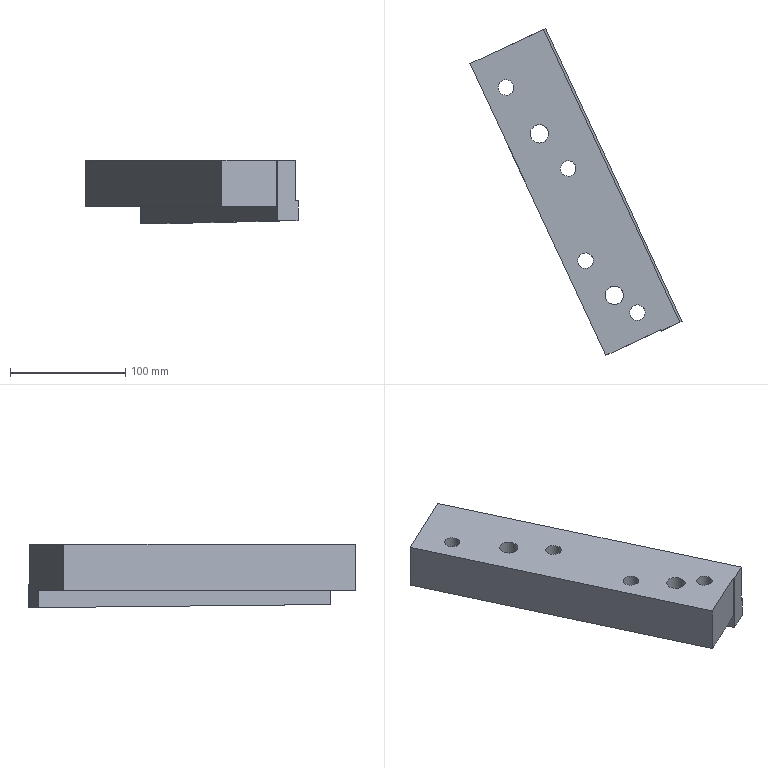Part | NX | features solid 2 | 1 solid | 25 faces | box 183.912 x 283.44 x 55 mm | volume 810388 mm3 | plane 15 | cylinder 10 | commonest cylinder face diameters 13.5 x4 19.5 x4 16 x2
STEP:
#1=CARTESIAN_POINT('',(122.71,137.916,3.));
#2=VERTEX_POINT('',#1);
#3=CARTESIAN_POINT('',(4.8,390.776,3.));
#4=VERTEX_POINT('',#3);
#5=CARTESIAN_POINT('',(204.661,-37.827,3.));
#6=DIRECTION('',(0.4226,-0.9063,0.));
#7=VECTOR('',#6,1000.);
#8=LINE('',#5,#7);
#9=EDGE_CURVE('',#2,#4,#8,.F.);
#10=ORIENTED_EDGE('',*,*,#9,.F.);
#11=CARTESIAN_POINT('',(122.71,137.916,43.));
#12=VERTEX_POINT('',#11);
#13=CARTESIAN_POINT('',(122.71,137.916,-107.));
#14=DIRECTION('',(0.,0.,1.));
#15=VECTOR('',#14,1000.);
#16=LINE('',#13,#15);
#17=EDGE_CURVE('',#2,#12,#16,.T.);
#18=ORIENTED_EDGE('',*,*,#17,.T.);
#19=CARTESIAN_POINT('',(4.8,390.776,43.));
#20=VERTEX_POINT('',#19);
#21=CARTESIAN_POINT('',(192.036,-10.753,43.));
#22=DIRECTION('',(0.4226,-0.9063,0.));
#23=VECTOR('',#22,1000.);
#24=LINE('',#21,#23);
#25=EDGE_CURVE('',#20,#12,#24,.T.);
#26=ORIENTED_EDGE('',*,*,#25,.F.);
#27=CARTESIAN_POINT('',(4.8,390.776,-107.));
#28=DIRECTION('',(0.,0.,-1.));
#29=VECTOR('',#28,1000.);
#30=LINE('',#27,#29);
#31=EDGE_CURVE('',#4,#20,#30,.F.);
#32=ORIENTED_EDGE('',*,*,#31,.F.);
#33=EDGE_LOOP('',(#10,#18,#26,#32));
#34=FACE_BOUND('',#33,.T.);
#35=CARTESIAN_POINT('',(215.,-60.,-107.));
#36=DIRECTION('',(-0.9063,-0.4226,0.));
#37=DIRECTION('',(-0.4226,0.9063,0.));
#38=AXIS2_PLACEMENT_3D('',#35,#36,#37);
#39=PLANE('',#38);
#40=ADVANCED_FACE('',(#34),#39,.T.);
#41=CARTESIAN_POINT('',(70.379,421.356,-12.));
#42=VERTEX_POINT('',#41);
#43=CARTESIAN_POINT('',(70.379,421.356,8.));
#44=VERTEX_POINT('',#43);
#45=CARTESIAN_POINT('',(70.379,421.356,-105.));
#46=DIRECTION('',(0.,0.,-1.));
#47=VECTOR('',#46,1000.);
#48=LINE('',#45,#47);
#49=EDGE_CURVE('',#42,#44,#48,.F.);
#50=ORIENTED_EDGE('',*,*,#49,.F.);
#51=CARTESIAN_POINT('',(52.252,412.903,-11.91));
#52=VERTEX_POINT('',#51);
#53=CARTESIAN_POINT('',(70.35,421.342,-12.));
#54=DIRECTION('',(-0.9063,-0.4226,0.004484));
#55=VECTOR('',#54,1000.);
#56=LINE('',#53,#55);
#57=EDGE_CURVE('',#42,#52,#56,.T.);
#58=ORIENTED_EDGE('',*,*,#57,.T.);
#59=CARTESIAN_POINT('',(52.252,412.903,3.));
#60=VERTEX_POINT('',#59);
#61=CARTESIAN_POINT('',(52.252,412.903,-5.));
#62=DIRECTION('',(0.,0.,1.));
#63=VECTOR('',#62,1000.);
#64=LINE('',#61,#63);
#65=EDGE_CURVE('',#60,#52,#64,.F.);
#66=ORIENTED_EDGE('',*,*,#65,.F.);
#67=CARTESIAN_POINT('',(-49.65,365.386,3.));
#68=DIRECTION('',(0.9063,0.4226,0.));
#69=VECTOR('',#68,1000.);
#70=LINE('',#67,#69);
#71=EDGE_CURVE('',#4,#60,#70,.T.);
#72=ORIENTED_EDGE('',*,*,#71,.F.);
#73=ORIENTED_EDGE('',*,*,#31,.T.);
#74=CARTESIAN_POINT('',(68.566,420.51,43.));
#75=VERTEX_POINT('',#74);
#76=CARTESIAN_POINT('',(204.565,483.928,43.));
#77=DIRECTION('',(0.9063,0.4226,0.));
#78=VECTOR('',#77,1000.);
#79=LINE('',#76,#78);
#80=EDGE_CURVE('',#20,#75,#79,.T.);
#81=ORIENTED_EDGE('',*,*,#80,.T.);
#82=CARTESIAN_POINT('',(68.566,420.51,8.));
#83=VERTEX_POINT('',#82);
#84=CARTESIAN_POINT('',(68.566,420.51,43.));
#85=DIRECTION('',(0.,0.,-1.));
#86=VECTOR('',#85,1000.);
#87=LINE('',#84,#86);
#88=EDGE_CURVE('',#83,#75,#87,.F.);
#89=ORIENTED_EDGE('',*,*,#88,.F.);
#90=CARTESIAN_POINT('',(-32.617,373.328,8.));
#91=DIRECTION('',(-0.9063,-0.4226,0.));
#92=VECTOR('',#91,1000.);
#93=LINE('',#90,#92);
#94=EDGE_CURVE('',#44,#83,#93,.T.);
#95=ORIENTED_EDGE('',*,*,#94,.F.);
#96=EDGE_LOOP('',(#50,#58,#66,#72,#73,#81,#89,#95));
#97=FACE_BOUND('',#96,.T.);
#98=CARTESIAN_POINT('',(70.379,421.356,-5.));
#99=DIRECTION('',(-0.4226,0.9063,0.));
#100=DIRECTION('',(0.,0.,-1.));
#101=AXIS2_PLACEMENT_3D('',#98,#99,#100);
#102=PLANE('',#101);
#103=ADVANCED_FACE('',(#97),#102,.T.);
#104=CARTESIAN_POINT('',(186.899,166.744,8.));
#105=VERTEX_POINT('',#104);
#106=CARTESIAN_POINT('',(81.245,393.321,8.));
#107=DIRECTION('',(-0.4226,0.9063,0.));
#108=VECTOR('',#107,1000.);
#109=LINE('',#106,#108);
#110=EDGE_CURVE('',#83,#105,#109,.F.);
#111=ORIENTED_EDGE('',*,*,#110,.F.);
#112=ORIENTED_EDGE('',*,*,#88,.T.);
#113=CARTESIAN_POINT('',(186.899,166.744,43.));
#114=VERTEX_POINT('',#113);
#115=CARTESIAN_POINT('',(81.245,393.321,43.));
#116=DIRECTION('',(-0.4226,0.9063,0.));
#117=VECTOR('',#116,1000.);
#118=LINE('',#115,#117);
#119=EDGE_CURVE('',#75,#114,#118,.F.);
#120=ORIENTED_EDGE('',*,*,#119,.T.);
#121=CARTESIAN_POINT('',(186.899,166.744,43.));
#122=DIRECTION('',(0.,0.,1.));
#123=VECTOR('',#122,1000.);
#124=LINE('',#121,#123);
#125=EDGE_CURVE('',#105,#114,#124,.T.);
#126=ORIENTED_EDGE('',*,*,#125,.F.);
#127=EDGE_LOOP('',(#111,#112,#120,#126));
#128=FACE_BOUND('',#127,.T.);
#129=CARTESIAN_POINT('',(81.245,393.321,43.));
#130=DIRECTION('',(-0.9063,-0.4226,0.));
#131=DIRECTION('',(-0.4226,0.9063,0.));
#132=AXIS2_PLACEMENT_3D('',#129,#130,#131);
#133=PLANE('',#132);
#134=ADVANCED_FACE('',(#128),#133,.F.);
#135=CARTESIAN_POINT('',(188.712,167.589,-9.308));
#136=VERTEX_POINT('',#135);
#137=CARTESIAN_POINT('',(281.198,-30.747,-7.203));
#138=DIRECTION('',(-0.4226,0.9063,-0.009616));
#139=VECTOR('',#138,1000.);
#140=LINE('',#137,#139);
#141=EDGE_CURVE('',#42,#136,#140,.F.);
#142=ORIENTED_EDGE('',*,*,#141,.F.);
#143=ORIENTED_EDGE('',*,*,#49,.T.);
#144=CARTESIAN_POINT('',(188.712,167.589,8.));
#145=VERTEX_POINT('',#144);
#146=CARTESIAN_POINT('',(178.495,189.499,8.));
#147=DIRECTION('',(-0.4226,0.9063,0.));
#148=VECTOR('',#147,1000.);
#149=LINE('',#146,#148);
#150=EDGE_CURVE('',#44,#145,#149,.F.);
#151=ORIENTED_EDGE('',*,*,#150,.T.);
#152=CARTESIAN_POINT('',(188.712,167.589,-105.));
#153=DIRECTION('',(0.,0.,1.));
#154=VECTOR('',#153,1000.);
#155=LINE('',#152,#154);
#156=EDGE_CURVE('',#136,#145,#155,.T.);
#157=ORIENTED_EDGE('',*,*,#156,.F.);
#158=EDGE_LOOP('',(#142,#143,#151,#157));
#159=FACE_BOUND('',#158,.T.);
#160=CARTESIAN_POINT('',(290.14,-49.924,-105.));
#161=DIRECTION('',(-0.9063,-0.4226,0.));
#162=DIRECTION('',(-0.4226,0.9063,0.));
#163=AXIS2_PLACEMENT_3D('',#160,#161,#162);
#164=PLANE('',#163);
#165=ADVANCED_FACE('',(#159),#164,.F.);
#166=ORIENTED_EDGE('',*,*,#150,.F.);
#167=ORIENTED_EDGE('',*,*,#94,.T.);
#168=ORIENTED_EDGE('',*,*,#110,.T.);
#169=CARTESIAN_POINT('',(85.717,119.562,8.));
#170=DIRECTION('',(0.9063,0.4226,0.));
#171=VECTOR('',#170,1000.);
#172=LINE('',#169,#171);
#173=EDGE_CURVE('',#145,#105,#172,.F.);
#174=ORIENTED_EDGE('',*,*,#173,.F.);
#175=EDGE_LOOP('',(#166,#167,#168,#174));
#176=FACE_BOUND('',#175,.T.);
#177=CARTESIAN_POINT('',(-40.145,389.473,8.));
#178=DIRECTION('',(0.,0.,1.));
#179=DIRECTION('',(0.08716,-0.9962,0.));
#180=AXIS2_PLACEMENT_3D('',#177,#178,#179);
#181=PLANE('',#180);
#182=ADVANCED_FACE('',(#176),#181,.T.);
#183=CARTESIAN_POINT('',(170.586,159.137,-9.218));
#184=VERTEX_POINT('',#183);
#185=CARTESIAN_POINT('',(170.586,159.137,43.));
#186=VERTEX_POINT('',#185);
#187=CARTESIAN_POINT('',(170.586,159.137,3.));
#188=DIRECTION('',(0.,0.,1.));
#189=VECTOR('',#188,1000.);
#190=LINE('',#187,#189);
#191=EDGE_CURVE('',#184,#186,#190,.T.);
#192=ORIENTED_EDGE('',*,*,#191,.T.);
#193=CARTESIAN_POINT('',(170.163,160.043,43.));
#194=VERTEX_POINT('',#193);
#195=CARTESIAN_POINT('',(64.931,385.714,43.));
#196=DIRECTION('',(0.4226,-0.9063,0.));
#197=VECTOR('',#196,1000.);
#198=LINE('',#195,#197);
#199=EDGE_CURVE('',#194,#186,#198,.T.);
#200=ORIENTED_EDGE('',*,*,#199,.F.);
#201=CARTESIAN_POINT('',(170.163,160.043,3.));
#202=VERTEX_POINT('',#201);
#203=CARTESIAN_POINT('',(170.163,160.043,3.));
#204=DIRECTION('',(0.,0.,-1.));
#205=VECTOR('',#204,1000.);
#206=LINE('',#203,#205);
#207=EDGE_CURVE('',#202,#194,#206,.F.);
#208=ORIENTED_EDGE('',*,*,#207,.F.);
#209=CARTESIAN_POINT('',(64.931,385.714,3.));
#210=DIRECTION('',(0.4226,-0.9063,0.));
#211=VECTOR('',#210,1000.);
#212=LINE('',#209,#211);
#213=EDGE_CURVE('',#60,#202,#212,.T.);
#214=ORIENTED_EDGE('',*,*,#213,.F.);
#215=ORIENTED_EDGE('',*,*,#65,.T.);
#216=CARTESIAN_POINT('',(263.071,-39.199,-7.114));
#217=DIRECTION('',(-0.4226,0.9063,-0.009616));
#218=VECTOR('',#217,1000.);
#219=LINE('',#216,#218);
#220=EDGE_CURVE('',#52,#184,#219,.F.);
#221=ORIENTED_EDGE('',*,*,#220,.T.);
#222=EDGE_LOOP('',(#192,#200,#208,#214,#215,#221));
#223=FACE_BOUND('',#222,.T.);
#224=CARTESIAN_POINT('',(64.931,385.714,3.));
#225=DIRECTION('',(-0.9063,-0.4226,0.));
#226=DIRECTION('',(-0.4226,0.9063,0.));
#227=AXIS2_PLACEMENT_3D('',#224,#225,#226);
#228=PLANE('',#227);
#229=ADVANCED_FACE('',(#223),#228,.T.);
#230=CARTESIAN_POINT('',(65.,322.,3.));
#231=VERTEX_POINT('',#230);
#232=CARTESIAN_POINT('',(65.,330.,3.));
#233=DIRECTION('',(0.,0.,-1.));
#234=DIRECTION('',(0.,-1.,0.));
#235=AXIS2_PLACEMENT_3D('',#232,#233,#234);
#236=CIRCLE('',#235,8.);
#237=EDGE_CURVE('',#231,#231,#236,.T.);
#238=ORIENTED_EDGE('',*,*,#237,.F.);
#239=EDGE_LOOP('',(#238));
#240=FACE_BOUND('',#239,.T.);
#241=CARTESIAN_POINT('',(130.,182.,3.));
#242=VERTEX_POINT('',#241);
#243=CARTESIAN_POINT('',(130.,190.,3.));
#244=DIRECTION('',(0.,0.,-1.));
#245=DIRECTION('',(0.,-1.,0.));
#246=AXIS2_PLACEMENT_3D('',#243,#244,#245);
#247=CIRCLE('',#246,8.);
#248=EDGE_CURVE('',#242,#242,#247,.T.);
#249=ORIENTED_EDGE('',*,*,#248,.F.);
#250=EDGE_LOOP('',(#249));
#251=FACE_BOUND('',#250,.T.);
#252=CARTESIAN_POINT('',(36.079,360.489,3.));
#253=VERTEX_POINT('',#252);
#254=CARTESIAN_POINT('',(36.079,370.239,3.));
#255=DIRECTION('',(0.,0.,-1.));
#256=DIRECTION('',(0.,-1.,0.));
#257=AXIS2_PLACEMENT_3D('',#254,#255,#256);
#258=CIRCLE('',#257,9.75);
#259=EDGE_CURVE('',#253,#253,#258,.T.);
#260=ORIENTED_EDGE('',*,*,#259,.F.);
#261=EDGE_LOOP('',(#260));
#262=FACE_BOUND('',#261,.T.);
#263=CARTESIAN_POINT('',(90.,290.25,3.));
#264=VERTEX_POINT('',#263);
#265=CARTESIAN_POINT('',(90.,300.,3.));
#266=DIRECTION('',(0.,0.,-1.));
#267=DIRECTION('',(0.,-1.,0.));
#268=AXIS2_PLACEMENT_3D('',#265,#266,#267);
#269=CIRCLE('',#268,9.75);
#270=EDGE_CURVE('',#264,#264,#269,.T.);
#271=ORIENTED_EDGE('',*,*,#270,.F.);
#272=EDGE_LOOP('',(#271));
#273=FACE_BOUND('',#272,.T.);
#274=CARTESIAN_POINT('',(105.,210.25,3.));
#275=VERTEX_POINT('',#274);
#276=CARTESIAN_POINT('',(105.,220.,3.));
#277=DIRECTION('',(0.,0.,-1.));
#278=DIRECTION('',(0.,-1.,0.));
#279=AXIS2_PLACEMENT_3D('',#276,#277,#278);
#280=CIRCLE('',#279,9.75);
#281=EDGE_CURVE('',#275,#275,#280,.T.);
#282=ORIENTED_EDGE('',*,*,#281,.F.);
#283=EDGE_LOOP('',(#282));
#284=FACE_BOUND('',#283,.T.);
#285=CARTESIAN_POINT('',(150.,165.25,3.));
#286=VERTEX_POINT('',#285);
#287=CARTESIAN_POINT('',(150.,175.,3.));
#288=DIRECTION('',(0.,0.,-1.));
#289=DIRECTION('',(0.,-1.,0.));
#290=AXIS2_PLACEMENT_3D('',#287,#288,#289);
#291=CIRCLE('',#290,9.75);
#292=EDGE_CURVE('',#286,#286,#291,.T.);
#293=ORIENTED_EDGE('',*,*,#292,.F.);
#294=EDGE_LOOP('',(#293));
#295=FACE_BOUND('',#294,.T.);
#296=ORIENTED_EDGE('',*,*,#213,.T.);
#297=CARTESIAN_POINT('',(123.617,138.339,3.));
#298=DIRECTION('',(0.9063,0.4226,0.));
#299=VECTOR('',#298,1000.);
#300=LINE('',#297,#299);
#301=EDGE_CURVE('',#202,#2,#300,.F.);
#302=ORIENTED_EDGE('',*,*,#301,.T.);
#303=ORIENTED_EDGE('',*,*,#9,.T.);
#304=ORIENTED_EDGE('',*,*,#71,.T.);
#305=EDGE_LOOP('',(#296,#302,#303,#304));
#306=FACE_BOUND('',#305,.T.);
#307=CARTESIAN_POINT('',(-60.069,387.73,3.));
#308=DIRECTION('',(0.,0.,-1.));
#309=DIRECTION('',(0.08716,-0.9962,0.));
#310=AXIS2_PLACEMENT_3D('',#307,#308,#309);
#311=PLANE('',#310);
#312=ADVANCED_FACE('',(#240,#251,#262,#273,#284,#295,#306),#311,.T.);
#313=ORIENTED_EDGE('',*,*,#199,.T.);
#314=CARTESIAN_POINT('',(322.898,230.162,43.));
#315=DIRECTION('',(-0.9063,-0.4226,0.));
#316=VECTOR('',#315,1000.);
#317=LINE('',#314,#316);
#318=EDGE_CURVE('',#186,#114,#317,.F.);
#319=ORIENTED_EDGE('',*,*,#318,.T.);
#320=ORIENTED_EDGE('',*,*,#119,.F.);
#321=ORIENTED_EDGE('',*,*,#80,.F.);
#322=ORIENTED_EDGE('',*,*,#25,.T.);
#323=CARTESIAN_POINT('',(123.617,138.339,43.));
#324=DIRECTION('',(0.9063,0.4226,0.));
#325=VECTOR('',#324,1000.);
#326=LINE('',#323,#325);
#327=EDGE_CURVE('',#194,#12,#326,.F.);
#328=ORIENTED_EDGE('',*,*,#327,.F.);
#329=EDGE_LOOP('',(#313,#319,#320,#321,#322,#328));
#330=FACE_BOUND('',#329,.T.);
#331=CARTESIAN_POINT('',(73.,330.,43.));
#332=VERTEX_POINT('',#331);
#333=CARTESIAN_POINT('',(65.,330.,43.));
#334=DIRECTION('',(0.,0.,1.));
#335=DIRECTION('',(1.,0.,0.));
#336=AXIS2_PLACEMENT_3D('',#333,#334,#335);
#337=CIRCLE('',#336,8.);
#338=EDGE_CURVE('',#332,#332,#337,.F.);
#339=ORIENTED_EDGE('',*,*,#338,.T.);
#340=EDGE_LOOP('',(#339));
#341=FACE_BOUND('',#340,.T.);
#342=CARTESIAN_POINT('',(138.,190.,43.));
#343=VERTEX_POINT('',#342);
#344=CARTESIAN_POINT('',(130.,190.,43.));
#345=DIRECTION('',(0.,0.,1.));
#346=DIRECTION('',(1.,0.,0.));
#347=AXIS2_PLACEMENT_3D('',#344,#345,#346);
#348=CIRCLE('',#347,8.);
#349=EDGE_CURVE('',#343,#343,#348,.F.);
#350=ORIENTED_EDGE('',*,*,#349,.T.);
#351=EDGE_LOOP('',(#350));
#352=FACE_BOUND('',#351,.T.);
#353=CARTESIAN_POINT('',(42.829,370.239,43.));
#354=VERTEX_POINT('',#353);
#355=CARTESIAN_POINT('',(36.079,370.239,43.));
#356=DIRECTION('',(0.,0.,1.));
#357=DIRECTION('',(1.,0.,0.));
#358=AXIS2_PLACEMENT_3D('',#355,#356,#357);
#359=CIRCLE('',#358,6.75);
#360=EDGE_CURVE('',#354,#354,#359,.F.);
#361=ORIENTED_EDGE('',*,*,#360,.T.);
#362=EDGE_LOOP('',(#361));
#363=FACE_BOUND('',#362,.T.);
#364=CARTESIAN_POINT('',(96.75,300.,43.));
#365=VERTEX_POINT('',#364);
#366=CARTESIAN_POINT('',(90.,300.,43.));
#367=DIRECTION('',(0.,0.,1.));
#368=DIRECTION('',(1.,0.,0.));
#369=AXIS2_PLACEMENT_3D('',#366,#367,#368);
#370=CIRCLE('',#369,6.75);
#371=EDGE_CURVE('',#365,#365,#370,.F.);
#372=ORIENTED_EDGE('',*,*,#371,.T.);
#373=EDGE_LOOP('',(#372));
#374=FACE_BOUND('',#373,.T.);
#375=CARTESIAN_POINT('',(111.75,220.,43.));
#376=VERTEX_POINT('',#375);
#377=CARTESIAN_POINT('',(105.,220.,43.));
#378=DIRECTION('',(0.,0.,1.));
#379=DIRECTION('',(1.,0.,0.));
#380=AXIS2_PLACEMENT_3D('',#377,#378,#379);
#381=CIRCLE('',#380,6.75);
#382=EDGE_CURVE('',#376,#376,#381,.F.);
#383=ORIENTED_EDGE('',*,*,#382,.T.);
#384=EDGE_LOOP('',(#383));
#385=FACE_BOUND('',#384,.T.);
#386=CARTESIAN_POINT('',(156.75,175.,43.));
#387=VERTEX_POINT('',#386);
#388=CARTESIAN_POINT('',(150.,175.,43.));
#389=DIRECTION('',(0.,0.,1.));
#390=DIRECTION('',(1.,0.,0.));
#391=AXIS2_PLACEMENT_3D('',#388,#389,#390);
#392=CIRCLE('',#391,6.75);
#393=EDGE_CURVE('',#387,#387,#392,.F.);
#394=ORIENTED_EDGE('',*,*,#393,.T.);
#395=EDGE_LOOP('',(#394));
#396=FACE_BOUND('',#395,.T.);
#397=CARTESIAN_POINT('',(383.563,100.064,43.));
#398=DIRECTION('',(0.,0.,-1.));
#399=DIRECTION('',(0.9962,0.08716,0.));
#400=AXIS2_PLACEMENT_3D('',#397,#398,#399);
#401=PLANE('',#400);
#402=ADVANCED_FACE('',(#330,#341,#352,#363,#374,#385,#396),#401,.F.);
#403=ORIENTED_EDGE('',*,*,#220,.F.);
#404=ORIENTED_EDGE('',*,*,#57,.F.);
#405=ORIENTED_EDGE('',*,*,#141,.T.);
#406=CARTESIAN_POINT('',(155.822,152.253,-9.145));
#407=DIRECTION('',(-0.9063,-0.4226,0.004484));
#408=VECTOR('',#407,1000.);
#409=LINE('',#406,#408);
#410=EDGE_CURVE('',#184,#136,#409,.F.);
#411=ORIENTED_EDGE('',*,*,#410,.F.);
#412=EDGE_LOOP('',(#403,#404,#405,#411));
#413=FACE_BOUND('',#412,.T.);
#414=CARTESIAN_POINT('',(240.127,-49.896,-7.));
#415=DIRECTION('',(0.,-0.01061,-0.9999));
#416=DIRECTION('',(0.,0.9999,-0.01061));
#417=AXIS2_PLACEMENT_3D('',#414,#415,#416);
#418=PLANE('',#417);
#419=ADVANCED_FACE('',(#413),#418,.T.);
#420=ORIENTED_EDGE('',*,*,#318,.F.);
#421=ORIENTED_EDGE('',*,*,#191,.F.);
#422=ORIENTED_EDGE('',*,*,#410,.T.);
#423=ORIENTED_EDGE('',*,*,#156,.T.);
#424=ORIENTED_EDGE('',*,*,#173,.T.);
#425=ORIENTED_EDGE('',*,*,#125,.T.);
#426=EDGE_LOOP('',(#420,#421,#422,#423,#424,#425));
#427=FACE_BOUND('',#426,.T.);
#428=CARTESIAN_POINT('',(155.922,152.3,15.5));
#429=DIRECTION('',(-0.4226,0.9063,0.));
#430=DIRECTION('',(0.9063,0.4226,0.));
#431=AXIS2_PLACEMENT_3D('',#428,#429,#430);
#432=PLANE('',#431);
#433=ADVANCED_FACE('',(#427),#432,.F.);
#434=ORIENTED_EDGE('',*,*,#393,.F.);
#435=EDGE_LOOP('',(#434));
#436=FACE_BOUND('',#435,.T.);
#437=CARTESIAN_POINT('',(150.,168.25,28.));
#438=VERTEX_POINT('',#437);
#439=CARTESIAN_POINT('',(150.,175.,28.));
#440=DIRECTION('',(0.,0.,-1.));
#441=DIRECTION('',(0.,-1.,0.));
#442=AXIS2_PLACEMENT_3D('',#439,#440,#441);
#443=CIRCLE('',#442,6.75);
#444=EDGE_CURVE('',#438,#438,#443,.T.);
#445=ORIENTED_EDGE('',*,*,#444,.T.);
#446=EDGE_LOOP('',(#445));
#447=FACE_BOUND('',#446,.T.);
#448=CARTESIAN_POINT('',(150.,175.,53.));
#449=DIRECTION('',(0.,0.,1.));
#450=DIRECTION('',(0.,-1.,0.));
#451=AXIS2_PLACEMENT_3D('',#448,#449,#450);
#452=CYLINDRICAL_SURFACE('',#451,6.75);
#453=ADVANCED_FACE('',(#436,#447),#452,.F.);
#454=ORIENTED_EDGE('',*,*,#444,.F.);
#455=EDGE_LOOP('',(#454));
#456=FACE_BOUND('',#455,.T.);
#457=CARTESIAN_POINT('',(150.,165.25,28.));
#458=VERTEX_POINT('',#457);
#459=CARTESIAN_POINT('',(150.,175.,28.));
#460=DIRECTION('',(0.,0.,-1.));
#461=DIRECTION('',(0.,-1.,0.));
#462=AXIS2_PLACEMENT_3D('',#459,#460,#461);
#463=CIRCLE('',#462,9.75);
#464=EDGE_CURVE('',#458,#458,#463,.T.);
#465=ORIENTED_EDGE('',*,*,#464,.T.);
#466=EDGE_LOOP('',(#465));
#467=FACE_BOUND('',#466,.T.);
#468=CARTESIAN_POINT('',(150.,175.,28.));
#469=DIRECTION('',(0.,0.,1.));
#470=DIRECTION('',(0.,-1.,0.));
#471=AXIS2_PLACEMENT_3D('',#468,#469,#470);
#472=PLANE('',#471);
#473=ADVANCED_FACE('',(#456,#467),#472,.F.);
#474=ORIENTED_EDGE('',*,*,#464,.F.);
#475=EDGE_LOOP('',(#474));
#476=FACE_BOUND('',#475,.T.);
#477=ORIENTED_EDGE('',*,*,#292,.T.);
#478=EDGE_LOOP('',(#477));
#479=FACE_BOUND('',#478,.T.);
#480=CARTESIAN_POINT('',(150.,175.,3.));
#481=DIRECTION('',(0.,0.,1.));
#482=DIRECTION('',(0.,-1.,0.));
#483=AXIS2_PLACEMENT_3D('',#480,#481,#482);
#484=CYLINDRICAL_SURFACE('',#483,9.75);
#485=ADVANCED_FACE('',(#476,#479),#484,.F.);
#486=ORIENTED_EDGE('',*,*,#382,.F.);
#487=EDGE_LOOP('',(#486));
#488=FACE_BOUND('',#487,.T.);
#489=CARTESIAN_POINT('',(105.,213.25,28.));
#490=VERTEX_POINT('',#489);
#491=CARTESIAN_POINT('',(105.,220.,28.));
#492=DIRECTION('',(0.,0.,-1.));
#493=DIRECTION('',(0.,-1.,0.));
#494=AXIS2_PLACEMENT_3D('',#491,#492,#493);
#495=CIRCLE('',#494,6.75);
#496=EDGE_CURVE('',#490,#490,#495,.T.);
#497=ORIENTED_EDGE('',*,*,#496,.T.);
#498=EDGE_LOOP('',(#497));
#499=FACE_BOUND('',#498,.T.);
#500=CARTESIAN_POINT('',(105.,220.,53.));
#501=DIRECTION('',(0.,0.,1.));
#502=DIRECTION('',(0.,-1.,0.));
#503=AXIS2_PLACEMENT_3D('',#500,#501,#502);
#504=CYLINDRICAL_SURFACE('',#503,6.75);
#505=ADVANCED_FACE('',(#488,#499),#504,.F.);
#506=ORIENTED_EDGE('',*,*,#496,.F.);
#507=EDGE_LOOP('',(#506));
#508=FACE_BOUND('',#507,.T.);
#509=CARTESIAN_POINT('',(105.,210.25,28.));
#510=VERTEX_POINT('',#509);
#511=CARTESIAN_POINT('',(105.,220.,28.));
#512=DIRECTION('',(0.,0.,-1.));
#513=DIRECTION('',(0.,-1.,0.));
#514=AXIS2_PLACEMENT_3D('',#511,#512,#513);
#515=CIRCLE('',#514,9.75);
#516=EDGE_CURVE('',#510,#510,#515,.T.);
#517=ORIENTED_EDGE('',*,*,#516,.T.);
#518=EDGE_LOOP('',(#517));
#519=FACE_BOUND('',#518,.T.);
#520=CARTESIAN_POINT('',(105.,220.,28.));
#521=DIRECTION('',(0.,0.,1.));
#522=DIRECTION('',(0.,-1.,0.));
#523=AXIS2_PLACEMENT_3D('',#520,#521,#522);
#524=PLANE('',#523);
#525=ADVANCED_FACE('',(#508,#519),#524,.F.);
#526=ORIENTED_EDGE('',*,*,#516,.F.);
#527=EDGE_LOOP('',(#526));
#528=FACE_BOUND('',#527,.T.);
#529=ORIENTED_EDGE('',*,*,#281,.T.);
#530=EDGE_LOOP('',(#529));
#531=FACE_BOUND('',#530,.T.);
#532=CARTESIAN_POINT('',(105.,220.,3.));
#533=DIRECTION('',(0.,0.,1.));
#534=DIRECTION('',(0.,-1.,0.));
#535=AXIS2_PLACEMENT_3D('',#532,#533,#534);
#536=CYLINDRICAL_SURFACE('',#535,9.75);
#537=ADVANCED_FACE('',(#528,#531),#536,.F.);
#538=ORIENTED_EDGE('',*,*,#371,.F.);
#539=EDGE_LOOP('',(#538));
#540=FACE_BOUND('',#539,.T.);
#541=CARTESIAN_POINT('',(90.,293.25,28.));
#542=VERTEX_POINT('',#541);
#543=CARTESIAN_POINT('',(90.,300.,28.));
#544=DIRECTION('',(0.,0.,-1.));
#545=DIRECTION('',(0.,-1.,0.));
#546=AXIS2_PLACEMENT_3D('',#543,#544,#545);
#547=CIRCLE('',#546,6.75);
#548=EDGE_CURVE('',#542,#542,#547,.T.);
#549=ORIENTED_EDGE('',*,*,#548,.T.);
#550=EDGE_LOOP('',(#549));
#551=FACE_BOUND('',#550,.T.);
#552=CARTESIAN_POINT('',(90.,300.,53.));
#553=DIRECTION('',(0.,0.,1.));
#554=DIRECTION('',(0.,-1.,0.));
#555=AXIS2_PLACEMENT_3D('',#552,#553,#554);
#556=CYLINDRICAL_SURFACE('',#555,6.75);
#557=ADVANCED_FACE('',(#540,#551),#556,.F.);
#558=ORIENTED_EDGE('',*,*,#548,.F.);
#559=EDGE_LOOP('',(#558));
#560=FACE_BOUND('',#559,.T.);
#561=CARTESIAN_POINT('',(90.,290.25,28.));
#562=VERTEX_POINT('',#561);
#563=CARTESIAN_POINT('',(90.,300.,28.));
#564=DIRECTION('',(0.,0.,-1.));
#565=DIRECTION('',(0.,-1.,0.));
#566=AXIS2_PLACEMENT_3D('',#563,#564,#565);
#567=CIRCLE('',#566,9.75);
#568=EDGE_CURVE('',#562,#562,#567,.T.);
#569=ORIENTED_EDGE('',*,*,#568,.T.);
#570=EDGE_LOOP('',(#569));
#571=FACE_BOUND('',#570,.T.);
#572=CARTESIAN_POINT('',(90.,300.,28.));
#573=DIRECTION('',(0.,0.,1.));
#574=DIRECTION('',(0.,-1.,0.));
#575=AXIS2_PLACEMENT_3D('',#572,#573,#574);
#576=PLANE('',#575);
#577=ADVANCED_FACE('',(#560,#571),#576,.F.);
#578=ORIENTED_EDGE('',*,*,#568,.F.);
#579=EDGE_LOOP('',(#578));
#580=FACE_BOUND('',#579,.T.);
#581=ORIENTED_EDGE('',*,*,#270,.T.);
#582=EDGE_LOOP('',(#581));
#583=FACE_BOUND('',#582,.T.);
#584=CARTESIAN_POINT('',(90.,300.,3.));
#585=DIRECTION('',(0.,0.,1.));
#586=DIRECTION('',(0.,-1.,0.));
#587=AXIS2_PLACEMENT_3D('',#584,#585,#586);
#588=CYLINDRICAL_SURFACE('',#587,9.75);
#589=ADVANCED_FACE('',(#580,#583),#588,.F.);
#590=ORIENTED_EDGE('',*,*,#360,.F.);
#591=EDGE_LOOP('',(#590));
#592=FACE_BOUND('',#591,.T.);
#593=CARTESIAN_POINT('',(36.079,363.489,28.));
#594=VERTEX_POINT('',#593);
#595=CARTESIAN_POINT('',(36.079,370.239,28.));
#596=DIRECTION('',(0.,0.,-1.));
#597=DIRECTION('',(0.,-1.,0.));
#598=AXIS2_PLACEMENT_3D('',#595,#596,#597);
#599=CIRCLE('',#598,6.75);
#600=EDGE_CURVE('',#594,#594,#599,.T.);
#601=ORIENTED_EDGE('',*,*,#600,.T.);
#602=EDGE_LOOP('',(#601));
#603=FACE_BOUND('',#602,.T.);
#604=CARTESIAN_POINT('',(36.079,370.239,53.));
#605=DIRECTION('',(0.,0.,1.));
#606=DIRECTION('',(0.,-1.,0.));
#607=AXIS2_PLACEMENT_3D('',#604,#605,#606);
#608=CYLINDRICAL_SURFACE('',#607,6.75);
#609=ADVANCED_FACE('',(#592,#603),#608,.F.);
#610=ORIENTED_EDGE('',*,*,#600,.F.);
#611=EDGE_LOOP('',(#610));
#612=FACE_BOUND('',#611,.T.);
#613=CARTESIAN_POINT('',(36.079,360.489,28.));
#614=VERTEX_POINT('',#613);
#615=CARTESIAN_POINT('',(36.079,370.239,28.));
#616=DIRECTION('',(0.,0.,-1.));
#617=DIRECTION('',(0.,-1.,0.));
#618=AXIS2_PLACEMENT_3D('',#615,#616,#617);
#619=CIRCLE('',#618,9.75);
#620=EDGE_CURVE('',#614,#614,#619,.T.);
#621=ORIENTED_EDGE('',*,*,#620,.T.);
#622=EDGE_LOOP('',(#621));
#623=FACE_BOUND('',#622,.T.);
#624=CARTESIAN_POINT('',(36.079,370.239,28.));
#625=DIRECTION('',(0.,0.,1.));
#626=DIRECTION('',(0.,-1.,0.));
#627=AXIS2_PLACEMENT_3D('',#624,#625,#626);
#628=PLANE('',#627);
#629=ADVANCED_FACE('',(#612,#623),#628,.F.);
#630=ORIENTED_EDGE('',*,*,#620,.F.);
#631=EDGE_LOOP('',(#630));
#632=FACE_BOUND('',#631,.T.);
#633=ORIENTED_EDGE('',*,*,#259,.T.);
#634=EDGE_LOOP('',(#633));
#635=FACE_BOUND('',#634,.T.);
#636=CARTESIAN_POINT('',(36.079,370.239,3.));
#637=DIRECTION('',(0.,0.,1.));
#638=DIRECTION('',(0.,-1.,0.));
#639=AXIS2_PLACEMENT_3D('',#636,#637,#638);
#640=CYLINDRICAL_SURFACE('',#639,9.75);
#641=ADVANCED_FACE('',(#632,#635),#640,.F.);
#642=ORIENTED_EDGE('',*,*,#349,.F.);
#643=EDGE_LOOP('',(#642));
#644=FACE_BOUND('',#643,.T.);
#645=ORIENTED_EDGE('',*,*,#248,.T.);
#646=EDGE_LOOP('',(#645));
#647=FACE_BOUND('',#646,.T.);
#648=CARTESIAN_POINT('',(130.,190.,3.));
#649=DIRECTION('',(0.,0.,1.));
#650=DIRECTION('',(0.,-1.,0.));
#651=AXIS2_PLACEMENT_3D('',#648,#649,#650);
#652=CYLINDRICAL_SURFACE('',#651,8.);
#653=ADVANCED_FACE('',(#644,#647),#652,.F.);
#654=ORIENTED_EDGE('',*,*,#338,.F.);
#655=EDGE_LOOP('',(#654));
#656=FACE_BOUND('',#655,.T.);
#657=ORIENTED_EDGE('',*,*,#237,.T.);
#658=EDGE_LOOP('',(#657));
#659=FACE_BOUND('',#658,.T.);
#660=CARTESIAN_POINT('',(65.,330.,3.));
#661=DIRECTION('',(0.,0.,1.));
#662=DIRECTION('',(0.,-1.,0.));
#663=AXIS2_PLACEMENT_3D('',#660,#661,#662);
#664=CYLINDRICAL_SURFACE('',#663,8.);
#665=ADVANCED_FACE('',(#656,#659),#664,.F.);
#666=ORIENTED_EDGE('',*,*,#301,.F.);
#667=ORIENTED_EDGE('',*,*,#207,.T.);
#668=ORIENTED_EDGE('',*,*,#327,.T.);
#669=ORIENTED_EDGE('',*,*,#17,.F.);
#670=EDGE_LOOP('',(#666,#667,#668,#669));
#671=FACE_BOUND('',#670,.T.);
#672=CARTESIAN_POINT('',(123.617,138.339,3.));
#673=DIRECTION('',(0.4226,-0.9063,0.));
#674=DIRECTION('',(0.9063,0.4226,0.));
#675=AXIS2_PLACEMENT_3D('',#672,#673,#674);
#676=PLANE('',#675);
#677=ADVANCED_FACE('',(#671),#676,.T.);
#678=CLOSED_SHELL('',(#40,#103,#134,#165,#182,#229,#312,#402,#419,#433,#453,#473,#485,#505,#525,#537,#557,#577,#589,#609,#629,#641,#653,#665,#677));
#679=MANIFOLD_SOLID_BREP('',#678);
#680=(LENGTH_UNIT()NAMED_UNIT(*)SI_UNIT(.MILLI.,.METRE.));
#681=UNCERTAINTY_MEASURE_WITH_UNIT(LENGTH_MEASURE(0.00001),#680,'','');
#682=(NAMED_UNIT(*)PLANE_ANGLE_UNIT()SI_UNIT($,.RADIAN.));
#683=(NAMED_UNIT(*)SI_UNIT($,.STERADIAN.)SOLID_ANGLE_UNIT());
#684=(GEOMETRIC_REPRESENTATION_CONTEXT(3)GLOBAL_UNCERTAINTY_ASSIGNED_CONTEXT((#681))GLOBAL_UNIT_ASSIGNED_CONTEXT((#680,#682,#683))REPRESENTATION_CONTEXT('',''));
#685=ADVANCED_BREP_SHAPE_REPRESENTATION('',(#679),#684);